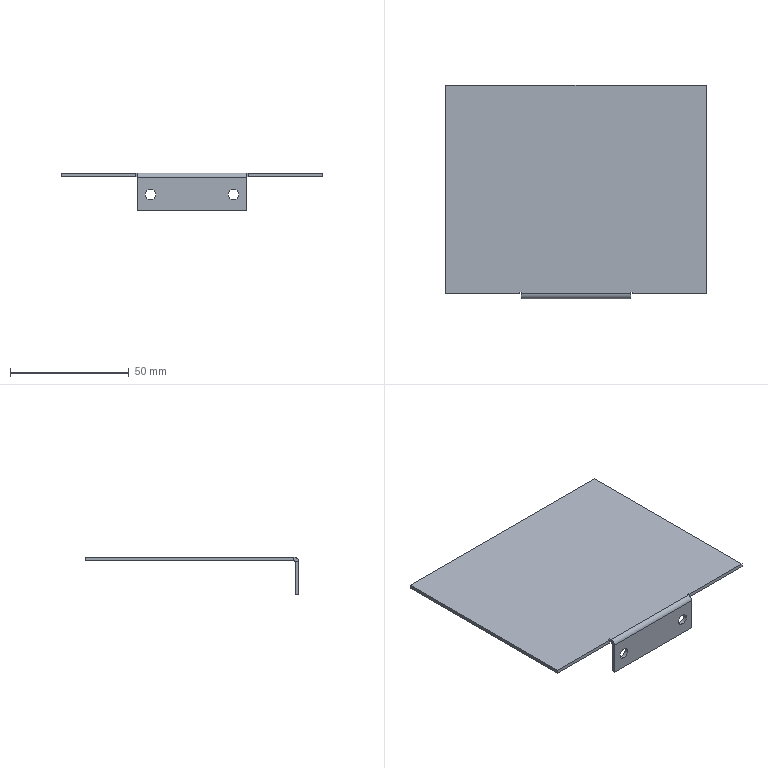Part | STEP file | B1-020 | 1 solid | 26 faces | box 110 x 90 x 16 mm | volume 15572 mm3 | plane 20 | cylinder 6 | commonest cylinder face diameters 4.5 x4 1 x1 4 x1